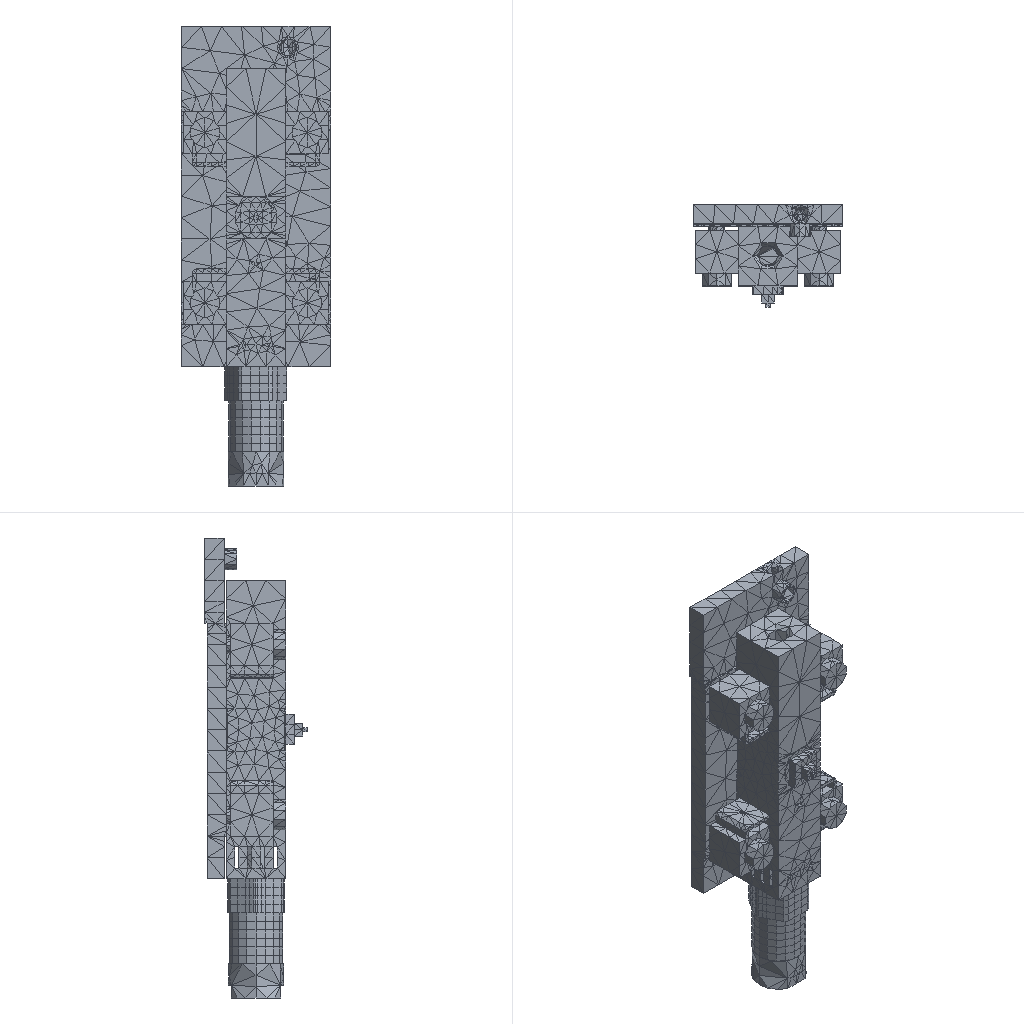Simulation study | ansys workbench
Set-up summary:
category,name,step,type,value,unit,region
solver,ansys_mapdl
solver,version,,,22.1
solver,version,,,22.1
units,MPA,,stated
analysis,deck1,,modal,HARM; modal
load_step,requested,,,3
analysis,nlgeom,,,False
mesh,nodes,,,20964
mesh,elements,,,13633
element_type,ANSYS 187 (type 1),,solid,4865
element_type,ANSYS 186 (type 2),,solid,35
element_type,ANSYS 186 (type 3),,solid,35
element_type,ANSYS 186 (type 4),,solid,35
element_type,ANSYS 186 (type 5),,solid,35
element_type,ANSYS 186 (type 6),,solid,35
element_type,ANSYS 186 (type 7),,solid,35
element_type,ANSYS 187 (type 8),,solid,296
element_type,ANSYS 186 (type 9),,solid,204
element_type,ANSYS 187 (type 10),,solid,621
element_type,ANSYS 186 (type 11),,solid,108
element_type,ANSYS 187 (type 12),,solid,2427
element_type,ANSYS 187 (type 13),,solid,146
element_type,ANSYS 187 (type 14),,solid,146
element_type,ANSYS 187 (type 15),,solid,146
element_type,ANSYS 187 (type 16),,solid,146
element_type,ANSYS 174 (type 17),,contact,100
element_type,ANSYS 170 (type 18),,target,100
element_type,ANSYS 174 (type 19),,contact,69
element_type,ANSYS 170 (type 20),,target,69
element_type,ANSYS 174 (type 21),,contact,193
element_type,ANSYS 170 (type 22),,target,193
element_type,ANSYS 174 (type 23),,contact,60
element_type,ANSYS 170 (type 24),,target,60
element_type,ANSYS 174 (type 25),,contact,358
element_type,ANSYS 170 (type 26),,target,358
element_type,ANSYS 174 (type 27),,contact,104
element_type,ANSYS 170 (type 28),,target,104
element_type,ANSYS 174 (type 29),,contact,104
element_type,ANSYS 170 (type 30),,target,104
element_type,ANSYS 174 (type 31),,contact,104
element_type,ANSYS 170 (type 32),,target,104
element_type,ANSYS 174 (type 33),,contact,104
element_type,ANSYS 170 (type 34),,target,104
element_type,ANSYS 174 (type 35),,contact,70
element_type,ANSYS 170 (type 36),,target,70
element_type,ANSYS 174 (type 37),,contact,70
element_type,ANSYS 170 (type 38),,target,70
element_type,ANSYS 174 (type 39),,contact,25
element_type,ANSYS 170 (type 40),,target,25
element_type,ANSYS 174 (type 41),,contact,70
element_type,ANSYS 170 (type 42),,target,70
element_type,ANSYS 174 (type 43),,contact,24
element_type,ANSYS 170 (type 44),,target,24
element_type,ANSYS 174 (type 45),,contact,75
element_type,ANSYS 170 (type 46),,target,75
element_type,ANSYS 174 (type 47),,contact,70
element_type,ANSYS 170 (type 48),,target,70
element_type,ANSYS 174 (type 49),,contact,28
element_type,ANSYS 170 (type 50),,target,28
element_type,ANSYS 174 (type 51),,contact,70
element_type,ANSYS 170 (type 52),,target,70
element_type,ANSYS 174 (type 53),,contact,28
element_type,ANSYS 170 (type 54),,target,28
element_type,ANSYS 174 (type 55),,contact,32
element_type,ANSYS 170 (type 56),,target,32
element_type,ANSYS 174 (type 57),,contact,86
element_type,ANSYS 170 (type 58),,target,86
element_type,ANSYS 174 (type 59),,contact,74
element_type,ANSYS 170 (type 60),,target,74
element_type,ANSYS 174 (type 61),,contact,111
element_type,ANSYS 170 (type 62),,target,111
element_type,ANSYS 154 (type 63),,surface,260
load,load commands in deck,,count,1
bc,support commands in deck,,count,0
analysis,deck2,,modal,modal
load_step,requested,,,1
analysis,nlgeom,,,False
mesh,nodes,,,20964
mesh,elements,,,13373
element_type,ANSYS 187 (type 1),,solid,4865
element_type,ANSYS 186 (type 2),,solid,35
element_type,ANSYS 186 (type 3),,solid,35
element_type,ANSYS 186 (type 4),,solid,35
element_type,ANSYS 186 (type 5),,solid,35
element_type,ANSYS 186 (type 6),,solid,35
element_type,ANSYS 186 (type 7),,solid,35
element_type,ANSYS 187 (type 8),,solid,296
element_type,ANSYS 186 (type 9),,solid,204
element_type,ANSYS 187 (type 10),,solid,621
element_type,ANSYS 186 (type 11),,solid,108
element_type,ANSYS 187 (type 12),,solid,2427
element_type,ANSYS 187 (type 13),,solid,146
element_type,ANSYS 187 (type 14),,solid,146
element_type,ANSYS 187 (type 15),,solid,146
element_type,ANSYS 187 (type 16),,solid,146
element_type,ANSYS 174 (type 17),,contact,100
element_type,ANSYS 170 (type 18),,target,100
element_type,ANSYS 174 (type 19),,contact,69
element_type,ANSYS 170 (type 20),,target,69
element_type,ANSYS 174 (type 21),,contact,193
element_type,ANSYS 170 (type 22),,target,193
element_type,ANSYS 174 (type 23),,contact,60
element_type,ANSYS 170 (type 24),,target,60
element_type,ANSYS 174 (type 25),,contact,358
element_type,ANSYS 170 (type 26),,target,358
element_type,ANSYS 174 (type 27),,contact,104
element_type,ANSYS 170 (type 28),,target,104
element_type,ANSYS 174 (type 29),,contact,104
element_type,ANSYS 170 (type 30),,target,104
element_type,ANSYS 174 (type 31),,contact,104
element_type,ANSYS 170 (type 32),,target,104
element_type,ANSYS 174 (type 33),,contact,104
element_type,ANSYS 170 (type 34),,target,104
element_type,ANSYS 174 (type 35),,contact,70
element_type,ANSYS 170 (type 36),,target,70
element_type,ANSYS 174 (type 37),,contact,70
element_type,ANSYS 170 (type 38),,target,70
element_type,ANSYS 174 (type 39),,contact,25
element_type,ANSYS 170 (type 40),,target,25
element_type,ANSYS 174 (type 41),,contact,70
element_type,ANSYS 170 (type 42),,target,70
element_type,ANSYS 174 (type 43),,contact,24
element_type,ANSYS 170 (type 44),,target,24
element_type,ANSYS 174 (type 45),,contact,75
element_type,ANSYS 170 (type 46),,target,75
element_type,ANSYS 174 (type 47),,contact,70
element_type,ANSYS 170 (type 48),,target,70
element_type,ANSYS 174 (type 49),,contact,28
element_type,ANSYS 170 (type 50),,target,28
element_type,ANSYS 174 (type 51),,contact,70
element_type,ANSYS 170 (type 52),,target,70
element_type,ANSYS 174 (type 53),,contact,28
element_type,ANSYS 170 (type 54),,target,28
element_type,ANSYS 174 (type 55),,contact,32
element_type,ANSYS 170 (type 56),,target,32
element_type,ANSYS 174 (type 57),,contact,86
element_type,ANSYS 170 (type 58),,target,86
element_type,ANSYS 174 (type 59),,contact,74
element_type,ANSYS 170 (type 60),,target,74
element_type,ANSYS 174 (type 61),,contact,111
element_type,ANSYS 170 (type 62),,target,111
load,load commands in deck,,count,0
bc,support commands in deck,,count,1
named_set,_FIXEDSU,,component
material,1,,in results
material,2,,in results
material,3,,in results
material,4,,in results
material,5,,in results
material,6,,in results
material,7,,in results
material,8,,in results
material,9,,in results
material,10,,in results
material,11,,in results
material,12,,in results
material,13,,in results
material,14,,in results
material,15,,in results
material,16,,in results
material,1,,in results
material,2,,in results
material,3,,in results
material,4,,in results
material,5,,in results
material,6,,in results
material,7,,in results
material,8,,in results
material,9,,in results
material,10,,in results
material,11,,in results
material,12,,in results
material,13,,in results
material,14,,in results
material,15,,in results
material,16,,in results
check,setup vs results,,match,260 surface effect element(s) are not in the reader's mesh and were not compared
check,setup vs results,,match
Results summary:
result,analysis,,,msup
result,last_loadstep,,,1
result,primary field,,,displacement
result,mass,,,0.000268,"NMM: mm, ton, N, s, mV, mA, degC"
result,analysis,,,modal
result,last_loadstep,,,1
result,primary field,,,displacement